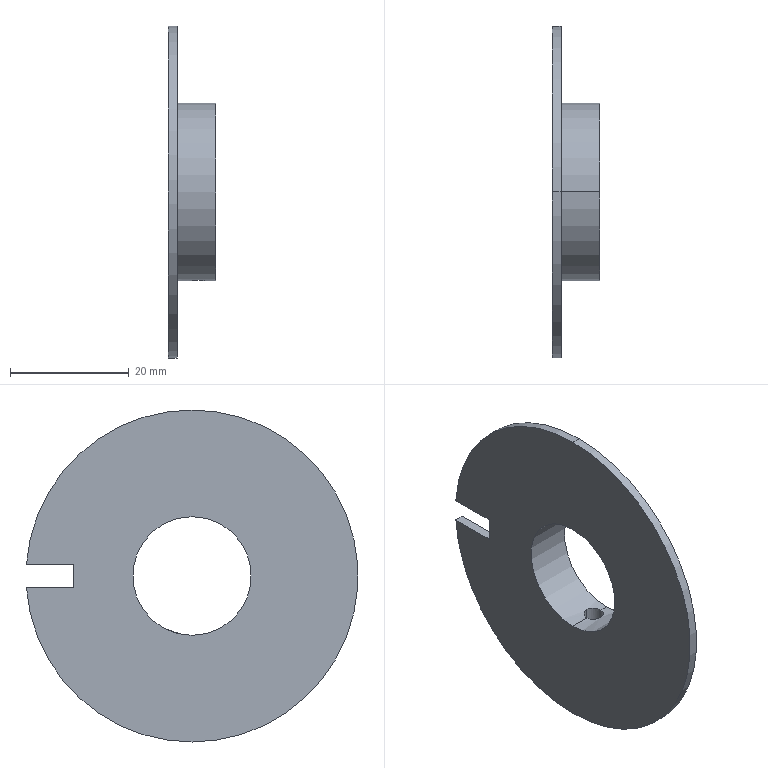Part | SolidWorks | features 3DProfileFeature 1, HoleWzd 1, ICE 1, Revolution 1 | 1 solid | 15 faces | box 8 x 55.928 x 56 mm | volume 5685 mm3 | cylinder 9 | plane 6 | commonest cylinder face diameters 56 x3 3.3 x2 20 x2 30 x2
STEP:
#1=CARTESIAN_POINT('',(5.,-1.65,-9.863));
#2=VERTEX_POINT('',#1);
#3=CARTESIAN_POINT('',(3.35,0.,-10.));
#4=VERTEX_POINT('',#3);
#5=CARTESIAN_POINT('',(5.,-1.65,-9.863));
#6=CARTESIAN_POINT('',(4.784,-1.65,-9.863));
#7=CARTESIAN_POINT('',(4.567,-1.607,-9.87));
#8=CARTESIAN_POINT('',(4.17,-1.442,-9.896));
#9=CARTESIAN_POINT('',(3.986,-1.319,-9.914));
#10=CARTESIAN_POINT('',(3.758,-1.091,-9.941));
#11=CARTESIAN_POINT('',(3.688,-1.006,-9.95));
#12=CARTESIAN_POINT('',(3.568,-0.8273,-9.966));
#13=CARTESIAN_POINT('',(3.518,-0.7326,-9.974));
#14=CARTESIAN_POINT('',(3.393,-0.4325,-9.993));
#15=CARTESIAN_POINT('',(3.35,-0.2181,-10.));
#16=CARTESIAN_POINT('',(3.35,0.,-10.));
#17=B_SPLINE_CURVE_WITH_KNOTS('',3,(#5,#6,#7,#8,#9,#10,#11,#12,#13,#14,#15,#16),.UNSPECIFIED.,.F.,.F.,(4,2,2,2,2,4),(0.005167,0.005814,0.00646,0.006783,0.007106,0.007752),.UNSPECIFIED.);
#18=EDGE_CURVE('',#2,#4,#17,.T.);
#19=ORIENTED_EDGE('',*,*,#18,.F.);
#20=CARTESIAN_POINT('',(5.,-1.65,-14.909));
#21=VERTEX_POINT('',#20);
#22=CARTESIAN_POINT('',(5.,-1.65,-15.));
#23=DIRECTION('',(0.,0.,-1.));
#24=VECTOR('',#23,1000.);
#25=LINE('',#22,#24);
#26=EDGE_CURVE('',#2,#21,#25,.T.);
#27=ORIENTED_EDGE('',*,*,#26,.T.);
#28=CARTESIAN_POINT('',(3.35,0.,-15.));
#29=VERTEX_POINT('',#28);
#30=CARTESIAN_POINT('',(3.35,0.,-15.));
#31=CARTESIAN_POINT('',(3.35,-0.1077,-15.));
#32=CARTESIAN_POINT('',(3.361,-0.2171,-14.999));
#33=CARTESIAN_POINT('',(3.403,-0.4287,-14.994));
#34=CARTESIAN_POINT('',(3.434,-0.5316,-14.991));
#35=CARTESIAN_POINT('',(3.517,-0.7314,-14.982));
#36=CARTESIAN_POINT('',(3.569,-0.8278,-14.977));
#37=CARTESIAN_POINT('',(3.688,-1.006,-14.966));
#38=CARTESIAN_POINT('',(3.756,-1.09,-14.961));
#39=CARTESIAN_POINT('',(3.91,-1.244,-14.949));
#40=CARTESIAN_POINT('',(3.994,-1.312,-14.943));
#41=CARTESIAN_POINT('',(4.172,-1.431,-14.932));
#42=CARTESIAN_POINT('',(4.269,-1.483,-14.927));
#43=CARTESIAN_POINT('',(4.468,-1.566,-14.918));
#44=CARTESIAN_POINT('',(4.571,-1.597,-14.915));
#45=CARTESIAN_POINT('',(4.783,-1.639,-14.91));
#46=CARTESIAN_POINT('',(4.892,-1.65,-14.909));
#47=CARTESIAN_POINT('',(5.,-1.65,-14.909));
#48=B_SPLINE_CURVE_WITH_KNOTS('',3,(#30,#31,#32,#33,#34,#35,#36,#37,#38,#39,#40,#41,#42,#43,#44,#45,#46,#47),.UNSPECIFIED.,.F.,.F.,(4,2,2,2,2,2,2,2,4),(0.002582,0.002904,0.003227,0.00355,0.003872,0.004195,0.004517,0.00484,0.005163),.UNSPECIFIED.);
#49=EDGE_CURVE('',#29,#21,#48,.T.);
#50=ORIENTED_EDGE('',*,*,#49,.F.);
#51=CARTESIAN_POINT('',(5.,1.65,-14.909));
#52=VERTEX_POINT('',#51);
#53=CARTESIAN_POINT('',(5.,1.65,-14.909));
#54=CARTESIAN_POINT('',(4.891,1.65,-14.909));
#55=CARTESIAN_POINT('',(4.784,1.639,-14.91));
#56=CARTESIAN_POINT('',(4.573,1.597,-14.915));
#57=CARTESIAN_POINT('',(4.468,1.566,-14.918));
#58=CARTESIAN_POINT('',(4.268,1.483,-14.927));
#59=CARTESIAN_POINT('',(4.173,1.432,-14.932));
#60=CARTESIAN_POINT('',(3.994,1.312,-14.943));
#61=CARTESIAN_POINT('',(3.909,1.242,-14.949));
#62=CARTESIAN_POINT('',(3.681,1.014,-14.966));
#63=CARTESIAN_POINT('',(3.558,0.83,-14.978));
#64=CARTESIAN_POINT('',(3.393,0.4328,-14.995));
#65=CARTESIAN_POINT('',(3.35,0.2155,-15.));
#66=CARTESIAN_POINT('',(3.35,0.,-15.));
#67=B_SPLINE_CURVE_WITH_KNOTS('',3,(#53,#54,#55,#56,#57,#58,#59,#60,#61,#62,#63,#64,#65,#66),.UNSPECIFIED.,.F.,.F.,(4,2,2,2,2,2,4),(0.,0.0003227,0.0006455,0.0009682,0.001291,0.001936,0.002582),.UNSPECIFIED.);
#68=EDGE_CURVE('',#52,#29,#67,.T.);
#69=ORIENTED_EDGE('',*,*,#68,.F.);
#70=CARTESIAN_POINT('',(5.,1.65,-9.863));
#71=VERTEX_POINT('',#70);
#72=CARTESIAN_POINT('',(5.,1.65,-15.));
#73=DIRECTION('',(0.,0.,-1.));
#74=VECTOR('',#73,1000.);
#75=LINE('',#72,#74);
#76=EDGE_CURVE('',#71,#52,#75,.T.);
#77=ORIENTED_EDGE('',*,*,#76,.F.);
#78=CARTESIAN_POINT('',(3.35,0.,-10.));
#79=CARTESIAN_POINT('',(3.35,0.109,-10.));
#80=CARTESIAN_POINT('',(3.361,0.2162,-9.998));
#81=CARTESIAN_POINT('',(3.403,0.4273,-9.991));
#82=CARTESIAN_POINT('',(3.435,0.5323,-9.986));
#83=CARTESIAN_POINT('',(3.517,0.7318,-9.974));
#84=CARTESIAN_POINT('',(3.568,0.8264,-9.966));
#85=CARTESIAN_POINT('',(3.688,1.006,-9.95));
#86=CARTESIAN_POINT('',(3.757,1.09,-9.941));
#87=CARTESIAN_POINT('',(3.985,1.318,-9.914));
#88=CARTESIAN_POINT('',(4.168,1.441,-9.896));
#89=CARTESIAN_POINT('',(4.565,1.606,-9.871));
#90=CARTESIAN_POINT('',(4.782,1.65,-9.863));
#91=CARTESIAN_POINT('',(5.,1.65,-9.863));
#92=B_SPLINE_CURVE_WITH_KNOTS('',3,(#78,#79,#80,#81,#82,#83,#84,#85,#86,#87,#88,#89,#90,#91),.UNSPECIFIED.,.F.,.F.,(4,2,2,2,2,2,4),(0.007752,0.008074,0.008397,0.00872,0.009043,0.009688,0.01033),.UNSPECIFIED.);
#93=EDGE_CURVE('',#4,#71,#92,.T.);
#94=ORIENTED_EDGE('',*,*,#93,.F.);
#95=EDGE_LOOP('',(#19,#27,#50,#69,#77,#94));
#96=FACE_OUTER_BOUND('',#95,.T.);
#97=CARTESIAN_POINT('',(5.,0.,-15.));
#98=DIRECTION('',(0.,0.,-1.));
#99=DIRECTION('',(0.,1.,0.));
#100=AXIS2_PLACEMENT_3D('',#97,#98,#99);
#101=CYLINDRICAL_SURFACE('',#100,1.65);
#102=ADVANCED_FACE('',(#96),#101,.F.);
#103=CARTESIAN_POINT('',(8.,0.,-10.));
#104=VERTEX_POINT('',#103);
#105=CARTESIAN_POINT('',(8.,0.,10.));
#106=VERTEX_POINT('',#105);
#107=CARTESIAN_POINT('',(8.,0.,0.));
#108=DIRECTION('',(-1.,0.,0.));
#109=DIRECTION('',(0.,0.,1.));
#110=AXIS2_PLACEMENT_3D('',#107,#108,#109);
#111=CIRCLE('',#110,10.);
#112=EDGE_CURVE('',#104,#106,#111,.T.);
#113=ORIENTED_EDGE('',*,*,#112,.F.);
#114=CARTESIAN_POINT('',(6.65,0.,-10.));
#115=VERTEX_POINT('',#114);
#116=CARTESIAN_POINT('',(0.,0.,-10.));
#117=DIRECTION('',(-1.,0.,0.));
#118=VECTOR('',#117,1000.);
#119=LINE('',#116,#118);
#120=EDGE_CURVE('',#104,#115,#119,.T.);
#121=ORIENTED_EDGE('',*,*,#120,.T.);
#122=CARTESIAN_POINT('',(6.65,0.,-10.));
#123=CARTESIAN_POINT('',(6.65,-0.1078,-10.));
#124=CARTESIAN_POINT('',(6.639,-0.2173,-9.998));
#125=CARTESIAN_POINT('',(6.597,-0.429,-9.991));
#126=CARTESIAN_POINT('',(6.566,-0.5319,-9.986));
#127=CARTESIAN_POINT('',(6.441,-0.8319,-9.967));
#128=CARTESIAN_POINT('',(6.32,-1.013,-9.95));
#129=CARTESIAN_POINT('',(6.09,-1.244,-9.923));
#130=CARTESIAN_POINT('',(6.007,-1.312,-9.914));
#131=CARTESIAN_POINT('',(5.828,-1.431,-9.897));
#132=CARTESIAN_POINT('',(5.731,-1.483,-9.89));
#133=CARTESIAN_POINT('',(5.532,-1.566,-9.877));
#134=CARTESIAN_POINT('',(5.429,-1.597,-9.872));
#135=CARTESIAN_POINT('',(5.217,-1.639,-9.865));
#136=CARTESIAN_POINT('',(5.108,-1.65,-9.863));
#137=CARTESIAN_POINT('',(5.,-1.65,-9.863));
#138=B_SPLINE_CURVE_WITH_KNOTS('',3,(#122,#123,#124,#125,#126,#127,#128,#129,#130,#131,#132,#133,#134,#135,#136,#137),.UNSPECIFIED.,.F.,.F.,(4,2,2,2,2,2,2,4),(0.002584,0.002907,0.00323,0.003876,0.004199,0.004522,0.004845,0.005167),.UNSPECIFIED.);
#139=EDGE_CURVE('',#115,#2,#138,.T.);
#140=ORIENTED_EDGE('',*,*,#139,.T.);
#141=ORIENTED_EDGE('',*,*,#18,.T.);
#142=CARTESIAN_POINT('',(0.,0.,-10.));
#143=VERTEX_POINT('',#142);
#144=CARTESIAN_POINT('',(0.,0.,-10.));
#145=DIRECTION('',(-1.,0.,0.));
#146=VECTOR('',#145,1000.);
#147=LINE('',#144,#146);
#148=EDGE_CURVE('',#4,#143,#147,.T.);
#149=ORIENTED_EDGE('',*,*,#148,.T.);
#150=CARTESIAN_POINT('',(0.,0.,10.));
#151=VERTEX_POINT('',#150);
#152=CARTESIAN_POINT('',(0.,0.,0.));
#153=DIRECTION('',(-1.,0.,0.));
#154=DIRECTION('',(0.,0.,1.));
#155=AXIS2_PLACEMENT_3D('',#152,#153,#154);
#156=CIRCLE('',#155,10.);
#157=EDGE_CURVE('',#143,#151,#156,.T.);
#158=ORIENTED_EDGE('',*,*,#157,.T.);
#159=CARTESIAN_POINT('',(0.,0.,10.));
#160=DIRECTION('',(-1.,0.,0.));
#161=VECTOR('',#160,1000.);
#162=LINE('',#159,#161);
#163=EDGE_CURVE('',#106,#151,#162,.T.);
#164=ORIENTED_EDGE('',*,*,#163,.F.);
#165=EDGE_LOOP('',(#113,#121,#140,#141,#149,#158,#164));
#166=FACE_OUTER_BOUND('',#165,.T.);
#167=CARTESIAN_POINT('',(0.,0.,0.));
#168=DIRECTION('',(-1.,0.,0.));
#169=DIRECTION('',(0.,0.,1.));
#170=AXIS2_PLACEMENT_3D('',#167,#168,#169);
#171=CYLINDRICAL_SURFACE('',#170,10.);
#172=ADVANCED_FACE('',(#166),#171,.F.);
#173=CARTESIAN_POINT('',(8.,0.,15.));
#174=VERTEX_POINT('',#173);
#175=CARTESIAN_POINT('',(8.,0.,-15.));
#176=VERTEX_POINT('',#175);
#177=CARTESIAN_POINT('',(8.,0.,0.));
#178=DIRECTION('',(-1.,0.,0.));
#179=DIRECTION('',(0.,0.,1.));
#180=AXIS2_PLACEMENT_3D('',#177,#178,#179);
#181=CIRCLE('',#180,15.);
#182=EDGE_CURVE('',#174,#176,#181,.T.);
#183=ORIENTED_EDGE('',*,*,#182,.T.);
#184=CARTESIAN_POINT('',(6.65,0.,-15.));
#185=VERTEX_POINT('',#184);
#186=CARTESIAN_POINT('',(0.,0.,-15.));
#187=DIRECTION('',(-1.,0.,0.));
#188=VECTOR('',#187,1000.);
#189=LINE('',#186,#188);
#190=EDGE_CURVE('',#176,#185,#189,.T.);
#191=ORIENTED_EDGE('',*,*,#190,.T.);
#192=CARTESIAN_POINT('',(6.65,0.,-15.));
#193=CARTESIAN_POINT('',(6.65,0.109,-15.));
#194=CARTESIAN_POINT('',(6.639,0.2163,-14.999));
#195=CARTESIAN_POINT('',(6.597,0.4271,-14.994));
#196=CARTESIAN_POINT('',(6.566,0.5319,-14.991));
#197=CARTESIAN_POINT('',(6.483,0.7316,-14.982));
#198=CARTESIAN_POINT('',(6.432,0.8263,-14.977));
#199=CARTESIAN_POINT('',(6.313,1.006,-14.967));
#200=CARTESIAN_POINT('',(6.243,1.09,-14.961));
#201=CARTESIAN_POINT('',(6.015,1.318,-14.943));
#202=CARTESIAN_POINT('',(5.831,1.441,-14.931));
#203=CARTESIAN_POINT('',(5.435,1.606,-14.914));
#204=CARTESIAN_POINT('',(5.218,1.65,-14.909));
#205=CARTESIAN_POINT('',(5.,1.65,-14.909));
#206=B_SPLINE_CURVE_WITH_KNOTS('',3,(#192,#193,#194,#195,#196,#197,#198,#199,#200,#201,#202,#203,#204,#205),.UNSPECIFIED.,.F.,.F.,(4,2,2,2,2,2,4),(0.007744,0.008067,0.008389,0.008712,0.009034,0.009679,0.01032),.UNSPECIFIED.);
#207=EDGE_CURVE('',#185,#52,#206,.T.);
#208=ORIENTED_EDGE('',*,*,#207,.T.);
#209=ORIENTED_EDGE('',*,*,#68,.T.);
#210=CARTESIAN_POINT('',(1.5,0.,-15.));
#211=VERTEX_POINT('',#210);
#212=CARTESIAN_POINT('',(0.,0.,-15.));
#213=DIRECTION('',(-1.,0.,0.));
#214=VECTOR('',#213,1000.);
#215=LINE('',#212,#214);
#216=EDGE_CURVE('',#29,#211,#215,.T.);
#217=ORIENTED_EDGE('',*,*,#216,.T.);
#218=CARTESIAN_POINT('',(1.5,0.,15.));
#219=VERTEX_POINT('',#218);
#220=CARTESIAN_POINT('',(1.5,0.,0.));
#221=DIRECTION('',(-1.,0.,0.));
#222=DIRECTION('',(0.,0.,1.));
#223=AXIS2_PLACEMENT_3D('',#220,#221,#222);
#224=CIRCLE('',#223,15.);
#225=EDGE_CURVE('',#219,#211,#224,.T.);
#226=ORIENTED_EDGE('',*,*,#225,.F.);
#227=CARTESIAN_POINT('',(0.,0.,15.));
#228=DIRECTION('',(-1.,0.,0.));
#229=VECTOR('',#228,1000.);
#230=LINE('',#227,#229);
#231=EDGE_CURVE('',#174,#219,#230,.T.);
#232=ORIENTED_EDGE('',*,*,#231,.F.);
#233=EDGE_LOOP('',(#183,#191,#208,#209,#217,#226,#232));
#234=FACE_OUTER_BOUND('',#233,.T.);
#235=CARTESIAN_POINT('',(0.,0.,0.));
#236=DIRECTION('',(-1.,0.,0.));
#237=DIRECTION('',(0.,0.,1.));
#238=AXIS2_PLACEMENT_3D('',#235,#236,#237);
#239=CYLINDRICAL_SURFACE('',#238,15.);
#240=ADVANCED_FACE('',(#234),#239,.T.);
#241=CARTESIAN_POINT('',(1.5,27.928,-2.));
#242=VERTEX_POINT('',#241);
#243=CARTESIAN_POINT('',(1.5,0.,-28.));
#244=VERTEX_POINT('',#243);
#245=CARTESIAN_POINT('',(1.5,0.,0.));
#246=DIRECTION('',(-1.,0.,0.));
#247=DIRECTION('',(0.,0.,1.));
#248=AXIS2_PLACEMENT_3D('',#245,#246,#247);
#249=CIRCLE('',#248,28.);
#250=EDGE_CURVE('',#242,#244,#249,.T.);
#251=ORIENTED_EDGE('',*,*,#250,.T.);
#252=CARTESIAN_POINT('',(0.,0.,-28.));
#253=VERTEX_POINT('',#252);
#254=CARTESIAN_POINT('',(0.,0.,-28.));
#255=DIRECTION('',(-1.,0.,0.));
#256=VECTOR('',#255,1000.);
#257=LINE('',#254,#256);
#258=EDGE_CURVE('',#244,#253,#257,.T.);
#259=ORIENTED_EDGE('',*,*,#258,.T.);
#260=CARTESIAN_POINT('',(0.,27.928,-2.));
#261=VERTEX_POINT('',#260);
#262=CARTESIAN_POINT('',(0.,0.,0.));
#263=DIRECTION('',(-1.,0.,0.));
#264=DIRECTION('',(0.,0.,1.));
#265=AXIS2_PLACEMENT_3D('',#262,#263,#264);
#266=CIRCLE('',#265,28.);
#267=EDGE_CURVE('',#261,#253,#266,.T.);
#268=ORIENTED_EDGE('',*,*,#267,.F.);
#269=CARTESIAN_POINT('',(0.,27.928,-2.));
#270=DIRECTION('',(-1.,0.,0.));
#271=VECTOR('',#270,1000.);
#272=LINE('',#269,#271);
#273=EDGE_CURVE('',#242,#261,#272,.T.);
#274=ORIENTED_EDGE('',*,*,#273,.F.);
#275=EDGE_LOOP('',(#251,#259,#268,#274));
#276=FACE_OUTER_BOUND('',#275,.T.);
#277=CARTESIAN_POINT('',(0.,0.,0.));
#278=DIRECTION('',(-1.,0.,0.));
#279=DIRECTION('',(0.,0.,1.));
#280=AXIS2_PLACEMENT_3D('',#277,#278,#279);
#281=CYLINDRICAL_SURFACE('',#280,28.);
#282=ADVANCED_FACE('',(#276),#281,.T.);
#283=ORIENTED_EDGE('',*,*,#258,.F.);
#284=CARTESIAN_POINT('',(1.5,0.,28.));
#285=VERTEX_POINT('',#284);
#286=CARTESIAN_POINT('',(1.5,0.,0.));
#287=DIRECTION('',(-1.,0.,0.));
#288=DIRECTION('',(0.,0.,1.));
#289=AXIS2_PLACEMENT_3D('',#286,#287,#288);
#290=CIRCLE('',#289,28.);
#291=EDGE_CURVE('',#244,#285,#290,.T.);
#292=ORIENTED_EDGE('',*,*,#291,.T.);
#293=CARTESIAN_POINT('',(0.,0.,28.));
#294=VERTEX_POINT('',#293);
#295=CARTESIAN_POINT('',(0.,0.,28.));
#296=DIRECTION('',(-1.,0.,0.));
#297=VECTOR('',#296,1000.);
#298=LINE('',#295,#297);
#299=EDGE_CURVE('',#285,#294,#298,.T.);
#300=ORIENTED_EDGE('',*,*,#299,.T.);
#301=CARTESIAN_POINT('',(0.,0.,0.));
#302=DIRECTION('',(-1.,0.,0.));
#303=DIRECTION('',(0.,0.,1.));
#304=AXIS2_PLACEMENT_3D('',#301,#302,#303);
#305=CIRCLE('',#304,28.);
#306=EDGE_CURVE('',#253,#294,#305,.T.);
#307=ORIENTED_EDGE('',*,*,#306,.F.);
#308=EDGE_LOOP('',(#283,#292,#300,#307));
#309=FACE_OUTER_BOUND('',#308,.T.);
#310=CARTESIAN_POINT('',(0.,0.,0.));
#311=DIRECTION('',(-1.,0.,0.));
#312=DIRECTION('',(0.,0.,1.));
#313=AXIS2_PLACEMENT_3D('',#310,#311,#312);
#314=CYLINDRICAL_SURFACE('',#313,28.);
#315=ADVANCED_FACE('',(#309),#314,.T.);
#316=CARTESIAN_POINT('',(0.,0.,0.));
#317=DIRECTION('',(-1.,0.,0.));
#318=DIRECTION('',(0.,0.,1.));
#319=AXIS2_PLACEMENT_3D('',#316,#317,#318);
#320=CIRCLE('',#319,10.);
#321=EDGE_CURVE('',#151,#143,#320,.T.);
#322=ORIENTED_EDGE('',*,*,#321,.F.);
#323=ORIENTED_EDGE('',*,*,#157,.F.);
#324=EDGE_LOOP('',(#322,#323));
#325=FACE_BOUND('',#324,.T.);
#326=CARTESIAN_POINT('',(0.,20.,-2.));
#327=VERTEX_POINT('',#326);
#328=CARTESIAN_POINT('',(0.,20.,2.));
#329=VERTEX_POINT('',#328);
#330=CARTESIAN_POINT('',(0.,20.,-2.));
#331=DIRECTION('',(0.,0.,1.));
#332=VECTOR('',#331,1000.);
#333=LINE('',#330,#332);
#334=EDGE_CURVE('',#327,#329,#333,.T.);
#335=ORIENTED_EDGE('',*,*,#334,.F.);
#336=CARTESIAN_POINT('',(0.,20.,-2.));
#337=DIRECTION('',(0.,-1.,0.));
#338=VECTOR('',#337,1000.);
#339=LINE('',#336,#338);
#340=EDGE_CURVE('',#261,#327,#339,.T.);
#341=ORIENTED_EDGE('',*,*,#340,.F.);
#342=ORIENTED_EDGE('',*,*,#267,.T.);
#343=ORIENTED_EDGE('',*,*,#306,.T.);
#344=CARTESIAN_POINT('',(0.,27.928,2.));
#345=VERTEX_POINT('',#344);
#346=CARTESIAN_POINT('',(0.,0.,0.));
#347=DIRECTION('',(-1.,0.,0.));
#348=DIRECTION('',(0.,0.,1.));
#349=AXIS2_PLACEMENT_3D('',#346,#347,#348);
#350=CIRCLE('',#349,28.);
#351=EDGE_CURVE('',#294,#345,#350,.T.);
#352=ORIENTED_EDGE('',*,*,#351,.T.);
#353=CARTESIAN_POINT('',(0.,20.,2.));
#354=DIRECTION('',(0.,1.,0.));
#355=VECTOR('',#354,1000.);
#356=LINE('',#353,#355);
#357=EDGE_CURVE('',#329,#345,#356,.T.);
#358=ORIENTED_EDGE('',*,*,#357,.F.);
#359=EDGE_LOOP('',(#335,#341,#342,#343,#352,#358));
#360=FACE_OUTER_BOUND('',#359,.T.);
#361=CARTESIAN_POINT('',(0.,10.,0.));
#362=DIRECTION('',(1.,0.,0.));
#363=DIRECTION('',(0.,0.,-1.));
#364=AXIS2_PLACEMENT_3D('',#361,#362,#363);
#365=PLANE('',#364);
#366=ADVANCED_FACE('',(#325,#360),#365,.F.);
#367=ORIENTED_EDGE('',*,*,#299,.F.);
#368=CARTESIAN_POINT('',(1.5,27.928,2.));
#369=VERTEX_POINT('',#368);
#370=CARTESIAN_POINT('',(1.5,0.,0.));
#371=DIRECTION('',(-1.,0.,0.));
#372=DIRECTION('',(0.,0.,1.));
#373=AXIS2_PLACEMENT_3D('',#370,#371,#372);
#374=CIRCLE('',#373,28.);
#375=EDGE_CURVE('',#285,#369,#374,.T.);
#376=ORIENTED_EDGE('',*,*,#375,.T.);
#377=CARTESIAN_POINT('',(0.,27.928,2.));
#378=DIRECTION('',(1.,0.,0.));
#379=VECTOR('',#378,1000.);
#380=LINE('',#377,#379);
#381=EDGE_CURVE('',#345,#369,#380,.T.);
#382=ORIENTED_EDGE('',*,*,#381,.F.);
#383=ORIENTED_EDGE('',*,*,#351,.F.);
#384=EDGE_LOOP('',(#367,#376,#382,#383));
#385=FACE_OUTER_BOUND('',#384,.T.);
#386=CARTESIAN_POINT('',(0.,0.,0.));
#387=DIRECTION('',(-1.,0.,0.));
#388=DIRECTION('',(0.,0.,1.));
#389=AXIS2_PLACEMENT_3D('',#386,#387,#388);
#390=CYLINDRICAL_SURFACE('',#389,28.);
#391=ADVANCED_FACE('',(#385),#390,.T.);
#392=ORIENTED_EDGE('',*,*,#250,.F.);
#393=CARTESIAN_POINT('',(1.5,20.,-2.));
#394=VERTEX_POINT('',#393);
#395=CARTESIAN_POINT('',(1.5,20.,-2.));
#396=DIRECTION('',(0.,1.,0.));
#397=VECTOR('',#396,1000.);
#398=LINE('',#395,#397);
#399=EDGE_CURVE('',#394,#242,#398,.T.);
#400=ORIENTED_EDGE('',*,*,#399,.F.);
#401=CARTESIAN_POINT('',(1.5,20.,2.));
#402=VERTEX_POINT('',#401);
#403=CARTESIAN_POINT('',(1.5,20.,-2.));
#404=DIRECTION('',(0.,0.,-1.));
#405=VECTOR('',#404,1000.);
#406=LINE('',#403,#405);
#407=EDGE_CURVE('',#402,#394,#406,.T.);
#408=ORIENTED_EDGE('',*,*,#407,.F.);
#409=CARTESIAN_POINT('',(1.5,20.,2.));
#410=DIRECTION('',(0.,-1.,0.));
#411=VECTOR('',#410,1000.);
#412=LINE('',#409,#411);
#413=EDGE_CURVE('',#369,#402,#412,.T.);
#414=ORIENTED_EDGE('',*,*,#413,.F.);
#415=ORIENTED_EDGE('',*,*,#375,.F.);
#416=ORIENTED_EDGE('',*,*,#291,.F.);
#417=EDGE_LOOP('',(#392,#400,#408,#414,#415,#416));
#418=FACE_OUTER_BOUND('',#417,.T.);
#419=ORIENTED_EDGE('',*,*,#225,.T.);
#420=CARTESIAN_POINT('',(1.5,0.,0.));
#421=DIRECTION('',(-1.,0.,0.));
#422=DIRECTION('',(0.,0.,1.));
#423=AXIS2_PLACEMENT_3D('',#420,#421,#422);
#424=CIRCLE('',#423,15.);
#425=EDGE_CURVE('',#211,#219,#424,.T.);
#426=ORIENTED_EDGE('',*,*,#425,.T.);
#427=EDGE_LOOP('',(#419,#426));
#428=FACE_BOUND('',#427,.T.);
#429=CARTESIAN_POINT('',(1.5,28.,0.));
#430=DIRECTION('',(-1.,0.,0.));
#431=DIRECTION('',(0.,0.,1.));
#432=AXIS2_PLACEMENT_3D('',#429,#430,#431);
#433=PLANE('',#432);
#434=ADVANCED_FACE('',(#418,#428),#433,.F.);
#435=ORIENTED_EDGE('',*,*,#190,.F.);
#436=CARTESIAN_POINT('',(8.,0.,0.));
#437=DIRECTION('',(-1.,0.,0.));
#438=DIRECTION('',(0.,0.,1.));
#439=AXIS2_PLACEMENT_3D('',#436,#437,#438);
#440=CIRCLE('',#439,15.);
#441=EDGE_CURVE('',#176,#174,#440,.T.);
#442=ORIENTED_EDGE('',*,*,#441,.T.);
#443=ORIENTED_EDGE('',*,*,#231,.T.);
#444=ORIENTED_EDGE('',*,*,#425,.F.);
#445=ORIENTED_EDGE('',*,*,#216,.F.);
#446=ORIENTED_EDGE('',*,*,#49,.T.);
#447=CARTESIAN_POINT('',(5.,-1.65,-14.909));
#448=CARTESIAN_POINT('',(5.216,-1.65,-14.909));
#449=CARTESIAN_POINT('',(5.433,-1.607,-14.914));
#450=CARTESIAN_POINT('',(5.83,-1.442,-14.931));
#451=CARTESIAN_POINT('',(6.014,-1.319,-14.943));
#452=CARTESIAN_POINT('',(6.242,-1.091,-14.96));
#453=CARTESIAN_POINT('',(6.312,-1.006,-14.966));
#454=CARTESIAN_POINT('',(6.432,-0.8269,-14.977));
#455=CARTESIAN_POINT('',(6.483,-0.7321,-14.982));
#456=CARTESIAN_POINT('',(6.566,-0.5323,-14.991));
#457=CARTESIAN_POINT('',(6.597,-0.4274,-14.994));
#458=CARTESIAN_POINT('',(6.639,-0.2164,-14.999));
#459=CARTESIAN_POINT('',(6.65,-0.1091,-15.));
#460=CARTESIAN_POINT('',(6.65,0.,-15.));
#461=B_SPLINE_CURVE_WITH_KNOTS('',3,(#447,#448,#449,#450,#451,#452,#453,#454,#455,#456,#457,#458,#459,#460),.UNSPECIFIED.,.F.,.F.,(4,2,2,2,2,2,4),(0.005163,0.005808,0.006453,0.006776,0.007099,0.007422,0.007744),.UNSPECIFIED.);
#462=EDGE_CURVE('',#21,#185,#461,.T.);
#463=ORIENTED_EDGE('',*,*,#462,.T.);
#464=EDGE_LOOP('',(#435,#442,#443,#444,#445,#446,#463));
#465=FACE_OUTER_BOUND('',#464,.T.);
#466=CARTESIAN_POINT('',(0.,0.,0.));
#467=DIRECTION('',(-1.,0.,0.));
#468=DIRECTION('',(0.,0.,1.));
#469=AXIS2_PLACEMENT_3D('',#466,#467,#468);
#470=CYLINDRICAL_SURFACE('',#469,15.);
#471=ADVANCED_FACE('',(#465),#470,.T.);
#472=ORIENTED_EDGE('',*,*,#182,.F.);
#473=ORIENTED_EDGE('',*,*,#441,.F.);
#474=EDGE_LOOP('',(#472,#473));
#475=FACE_OUTER_BOUND('',#474,.T.);
#476=CARTESIAN_POINT('',(8.,0.,0.));
#477=DIRECTION('',(-1.,0.,0.));
#478=DIRECTION('',(0.,0.,1.));
#479=AXIS2_PLACEMENT_3D('',#476,#477,#478);
#480=CIRCLE('',#479,10.);
#481=EDGE_CURVE('',#106,#104,#480,.T.);
#482=ORIENTED_EDGE('',*,*,#481,.T.);
#483=ORIENTED_EDGE('',*,*,#112,.T.);
#484=EDGE_LOOP('',(#482,#483));
#485=FACE_BOUND('',#484,.T.);
#486=CARTESIAN_POINT('',(8.,10.,0.));
#487=DIRECTION('',(-1.,0.,0.));
#488=DIRECTION('',(0.,0.,1.));
#489=AXIS2_PLACEMENT_3D('',#486,#487,#488);
#490=PLANE('',#489);
#491=ADVANCED_FACE('',(#475,#485),#490,.F.);
#492=ORIENTED_EDGE('',*,*,#120,.F.);
#493=ORIENTED_EDGE('',*,*,#481,.F.);
#494=ORIENTED_EDGE('',*,*,#163,.T.);
#495=ORIENTED_EDGE('',*,*,#321,.T.);
#496=ORIENTED_EDGE('',*,*,#148,.F.);
#497=ORIENTED_EDGE('',*,*,#93,.T.);
#498=CARTESIAN_POINT('',(5.,1.65,-9.863));
#499=CARTESIAN_POINT('',(5.109,1.65,-9.863));
#500=CARTESIAN_POINT('',(5.217,1.639,-9.865));
#501=CARTESIAN_POINT('',(5.428,1.597,-9.872));
#502=CARTESIAN_POINT('',(5.533,1.565,-9.877));
#503=CARTESIAN_POINT('',(5.733,1.482,-9.89));
#504=CARTESIAN_POINT('',(5.827,1.432,-9.897));
#505=CARTESIAN_POINT('',(6.007,1.312,-9.914));
#506=CARTESIAN_POINT('',(6.091,1.242,-9.923));
#507=CARTESIAN_POINT('',(6.319,1.014,-9.95));
#508=CARTESIAN_POINT('',(6.442,0.8303,-9.967));
#509=CARTESIAN_POINT('',(6.607,0.4332,-9.993));
#510=CARTESIAN_POINT('',(6.65,0.2157,-10.));
#511=CARTESIAN_POINT('',(6.65,0.,-10.));
#512=B_SPLINE_CURVE_WITH_KNOTS('',3,(#498,#499,#500,#501,#502,#503,#504,#505,#506,#507,#508,#509,#510,#511),.UNSPECIFIED.,.F.,.F.,(4,2,2,2,2,2,4),(0.,0.000323,0.0006461,0.0009691,0.001292,0.001938,0.002584),.UNSPECIFIED.);
#513=EDGE_CURVE('',#71,#115,#512,.T.);
#514=ORIENTED_EDGE('',*,*,#513,.T.);
#515=EDGE_LOOP('',(#492,#493,#494,#495,#496,#497,#514));
#516=FACE_OUTER_BOUND('',#515,.T.);
#517=CARTESIAN_POINT('',(0.,0.,0.));
#518=DIRECTION('',(-1.,0.,0.));
#519=DIRECTION('',(0.,0.,1.));
#520=AXIS2_PLACEMENT_3D('',#517,#518,#519);
#521=CYLINDRICAL_SURFACE('',#520,10.);
#522=ADVANCED_FACE('',(#516),#521,.F.);
#523=ORIENTED_EDGE('',*,*,#273,.T.);
#524=ORIENTED_EDGE('',*,*,#340,.T.);
#525=CARTESIAN_POINT('',(8.001,20.,-2.));
#526=DIRECTION('',(-1.,0.,0.));
#527=VECTOR('',#526,1000.);
#528=LINE('',#525,#527);
#529=EDGE_CURVE('',#394,#327,#528,.T.);
#530=ORIENTED_EDGE('',*,*,#529,.F.);
#531=ORIENTED_EDGE('',*,*,#399,.T.);
#532=EDGE_LOOP('',(#523,#524,#530,#531));
#533=FACE_OUTER_BOUND('',#532,.T.);
#534=CARTESIAN_POINT('',(8.001,20.,-2.));
#535=DIRECTION('',(0.,0.,-1.));
#536=DIRECTION('',(-1.,0.,0.));
#537=AXIS2_PLACEMENT_3D('',#534,#535,#536);
#538=PLANE('',#537);
#539=ADVANCED_FACE('',(#533),#538,.F.);
#540=ORIENTED_EDGE('',*,*,#381,.T.);
#541=ORIENTED_EDGE('',*,*,#413,.T.);
#542=CARTESIAN_POINT('',(8.001,20.,2.));
#543=DIRECTION('',(-1.,0.,0.));
#544=VECTOR('',#543,1000.);
#545=LINE('',#542,#544);
#546=EDGE_CURVE('',#402,#329,#545,.T.);
#547=ORIENTED_EDGE('',*,*,#546,.T.);
#548=ORIENTED_EDGE('',*,*,#357,.T.);
#549=EDGE_LOOP('',(#540,#541,#547,#548));
#550=FACE_OUTER_BOUND('',#549,.T.);
#551=CARTESIAN_POINT('',(8.001,20.,2.));
#552=DIRECTION('',(0.,0.,1.));
#553=DIRECTION('',(1.,0.,0.));
#554=AXIS2_PLACEMENT_3D('',#551,#552,#553);
#555=PLANE('',#554);
#556=ADVANCED_FACE('',(#550),#555,.F.);
#557=ORIENTED_EDGE('',*,*,#407,.T.);
#558=ORIENTED_EDGE('',*,*,#529,.T.);
#559=ORIENTED_EDGE('',*,*,#334,.T.);
#560=ORIENTED_EDGE('',*,*,#546,.F.);
#561=EDGE_LOOP('',(#557,#558,#559,#560));
#562=FACE_OUTER_BOUND('',#561,.T.);
#563=CARTESIAN_POINT('',(8.001,20.,-2.));
#564=DIRECTION('',(0.,-1.,0.));
#565=DIRECTION('',(0.,0.,-1.));
#566=AXIS2_PLACEMENT_3D('',#563,#564,#565);
#567=PLANE('',#566);
#568=ADVANCED_FACE('',(#562),#567,.F.);
#569=ORIENTED_EDGE('',*,*,#26,.F.);
#570=ORIENTED_EDGE('',*,*,#139,.F.);
#571=ORIENTED_EDGE('',*,*,#513,.F.);
#572=ORIENTED_EDGE('',*,*,#76,.T.);
#573=ORIENTED_EDGE('',*,*,#207,.F.);
#574=ORIENTED_EDGE('',*,*,#462,.F.);
#575=EDGE_LOOP('',(#569,#570,#571,#572,#573,#574));
#576=FACE_OUTER_BOUND('',#575,.T.);
#577=CARTESIAN_POINT('',(5.,0.,-15.));
#578=DIRECTION('',(0.,0.,-1.));
#579=DIRECTION('',(0.,1.,0.));
#580=AXIS2_PLACEMENT_3D('',#577,#578,#579);
#581=CYLINDRICAL_SURFACE('',#580,1.65);
#582=ADVANCED_FACE('',(#576),#581,.F.);
#583=CLOSED_SHELL('',(#102,#172,#240,#282,#315,#366,#391,#434,#471,#491,#522,#539,#556,#568,#582));
#584=MANIFOLD_SOLID_BREP('',#583);
#585=CARTESIAN_POINT('',(0.,0.,0.));
#586=DIRECTION('',(0.,0.,1.));
#587=DIRECTION('',(1.,0.,0.));
#588=AXIS2_PLACEMENT_3D('',#585,#586,#587);
#589=(LENGTH_UNIT()NAMED_UNIT(*)SI_UNIT(.MILLI.,.METRE.));
#590=UNCERTAINTY_MEASURE_WITH_UNIT(LENGTH_MEASURE(0.00001),#589,'','');
#591=(NAMED_UNIT(*)PLANE_ANGLE_UNIT()SI_UNIT($,.RADIAN.));
#592=(NAMED_UNIT(*)SI_UNIT($,.STERADIAN.)SOLID_ANGLE_UNIT());
#593=(GEOMETRIC_REPRESENTATION_CONTEXT(3)GLOBAL_UNCERTAINTY_ASSIGNED_CONTEXT((#590))GLOBAL_UNIT_ASSIGNED_CONTEXT((#589,#591,#592))REPRESENTATION_CONTEXT('',''));
#594=ADVANCED_BREP_SHAPE_REPRESENTATION('',(#584,#588),#593);